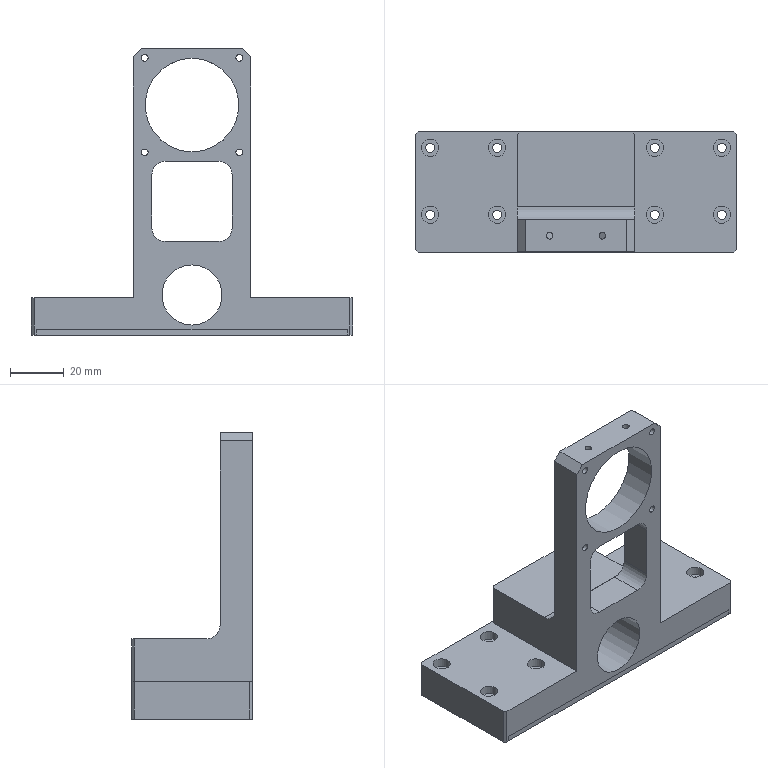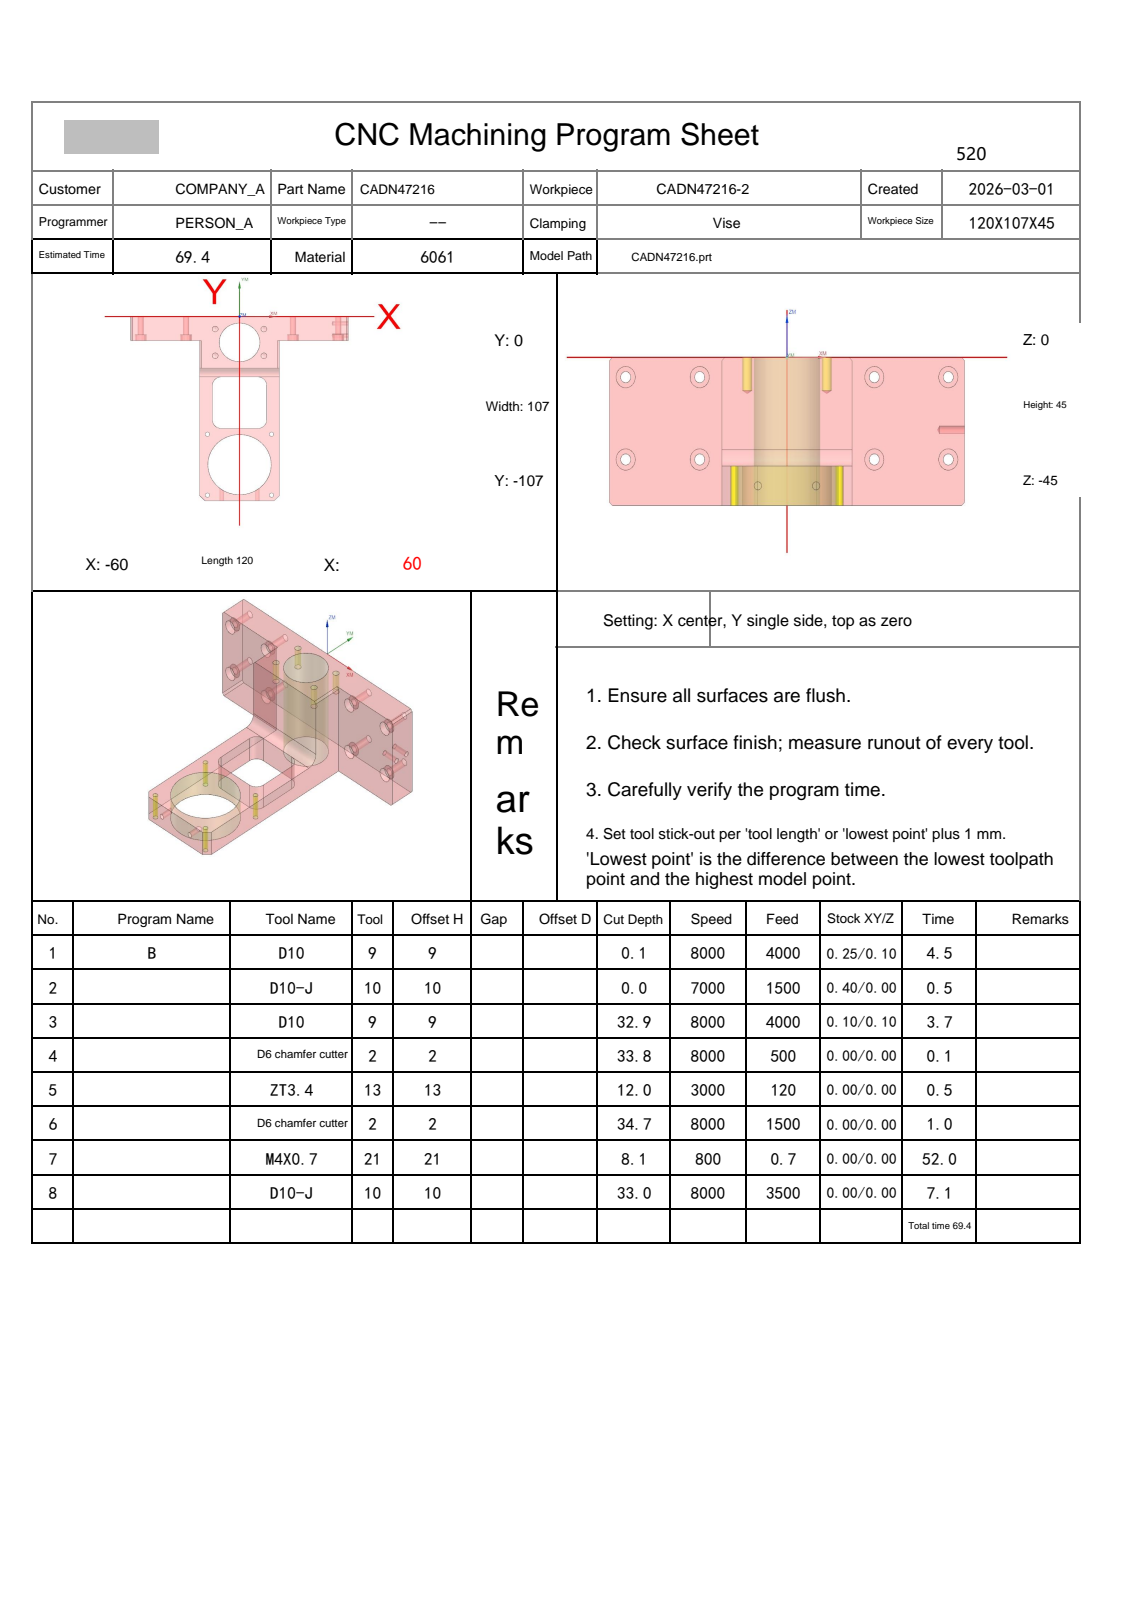NC program | NX | posted by the shop | part box 120 x 45 x 107 mm
Lines 1757 to 2535 of 8568:
N3 T09 M06
(D10  D=10. R=0. H=09 ce=0.10 di=0.10)
G00 G90 G54 X31.378 Y-24.062 M03 S8000
G43 H09 Z50.
M08
Z-14.45
G01 X31.287 Y-24.104 Z-15.075 F4000.
X31.196 Y-24.146 Z-15.322
X31.106 Y-24.188 Z-15.504
X31.015 Y-24.23 Z-15.65
X30.924 Y-24.273 Z-15.773
X30.834 Y-24.315 Z-15.878
X30.743 Y-24.357 Z-15.97
X30.652 Y-24.399 Z-16.05
X30.562 Y-24.441 Z-16.12
X30.471 Y-24.484 Z-16.182
X30.38 Y-24.526 Z-16.236
X30.29 Y-24.568 Z-16.283
X30.199 Y-24.61 Z-16.324
X30.108 Y-24.652 Z-16.358
X30.018 Y-24.695 Z-16.386
X29.927 Y-24.737 Z-16.41
X29.836 Y-24.779 Z-16.427
X29.746 Y-24.821 Z-16.44
X29.655 Y-24.863 Z-16.447
X29.564 Y-24.905 Z-16.45
X27.405 Y-25.91
G03 X27.113 Y-26.369 I.214 J-.458
G01 X27.151 Y-26.562
G02 X29.467 Y-30.08 I-25.429 J-19.261
X30.973 Y-36.095 I-14.623 J-6.857
X31.232 Y-44.397 I-132.782 J-8.303
X31.223 Y-46.009 I-133.041 J0.0
G01 X31.225 Y-102.469
G02 X28.237 Y-110.318 I-12.757 J.363
X23.784 Y-114.408 I-11.871 J8.455
X17.95 Y-115.972 I-6.708 J13.363
X9.211 Y-116.264 I-8.739 J130.435
X7.077 Y-116.247 I0.0 J130.728
G01 X-17.303 Y-116.232
G02 X-25.268 Y-113.271 I.206 J12.75
X-29.344 Y-108.898 I8.605 J12.105
X-30.935 Y-103.316 I12.645 J6.621
X-31.252 Y-95.378 I99.044 J7.938
X-31.242 Y-93.965 I99.361 J0.0
G01 X-31.225 Y-37.19
G02 X-31.229 Y-36.904 I11.714 J.286
X-29.463 Y-30.719 I11.718 J0.0
X-27.184 Y-28.116 I13.292 J-9.337
G01 X-27.1 Y-27.88
Y-26.52
X-27.126 Y-28.038
X-28.84 Y-31.056
G03 X-30.423 Y-37.625 I15.495 J-7.21
X-30.626 Y-46.505 I194. J-8.88
X-30.608 Y-49.142 I194.203 J0.0
G01 X-30.585 Y-96.082
G03 X-30.591 Y-96.853 I51.642 J-.771
X-30.097 Y-103.978 I51.647 J0.0
X-25.324 Y-112.093 I13.34 J2.385
X-17.597 Y-115.308 I8.755 J10.148
X-10.151 Y-115.615 I7.447 J90.294
X-8.726 Y-115.604 I0.0 J90.6
G01 X11.574 Y-115.579
G03 X12.22 Y-115.583 I.646 J46.187
X19.226 Y-115.049 I0.0 J46.192
X27.093 Y-110.328 I-2.634 J13.305
X30.314 Y-102.544 I-10.197 J8.777
X30.611 Y-95.169 I-91.526 J7.375
X30.6 Y-93.753 I-91.822 J0.0
G01 X30.561 Y-42.733
G03 X30.567 Y-41.955 I-52.094 J.778
X30.067 Y-34.756 I-52.1 J0.0
X27.429 Y-28.654 I-12.773 J-1.901
G02 X27.1 Y-28.125 I.757 J.838
G01 Y-26.525
X27.109 Y-28.284
G02 X28.595 Y-32.651 I-100.066 J-36.506
X29.677 Y-41.203 I-36.109 J-8.913
X29.793 Y-52.445 I-544.946 J-11.242
X29.789 Y-54.562 I-545.062 J0.0
G01 X29.778 Y-96.142
G02 X29.782 Y-96.738 I-41.25 J-.595
X29.28 Y-103.155 I-41.254 J0.0
X18.117 Y-114.102 I-13.308 J2.406
X10.092 Y-114.76 I-8.025 J48.608
G01 X9.834 Y-114.759
G02 X-.605 Y-114.831 I-10.439 J751.569
X-13.845 Y-114.715 I0.0 J751.641
X-20.222 Y-113.721 I.088 J21.521
X-29.054 Y-103.354 I4.381 J12.677
X-29.76 Y-95.187 I46.884 J8.167
X-29.759 Y-94.835 I47.59 J0.0
G01 X-29.809 Y-83.635
X-29.78 Y-42.775
G02 X-29.785 Y-42.143 I39.535 J.632
X-29.214 Y-35.448 I39.54 J0.0
X-27.14 Y-29.947 I23.047 J-5.549
G03 X-27.077 Y-28.644 I-13.57 J1.302
X-27.1 Y-27.857 I-13.632 J0.0
G02 X-27.077 Y-28.705 I-15.592 J-.848
X-27.165 Y-30.362 I-15.615 J0.0
G03 X-28.366 Y-34.989 I173.965 J-47.627
X-29.123 Y-43.529 I47.78 J-8.54
G01 X-29.122 Y-43.824
X-29.168 Y-53.664
X-29.144 Y-92.524
G03 X-29.148 Y-93.262 I66.05 J-.739
X-28.637 Y-101.462 I66.055 J0.0
X-25.247 Y-109.202 I14.471 J1.725
X-16.817 Y-113.605 I10.331 J9.509
X-8.943 Y-114.149 I7.873 J56.692
X-8.202 Y-114.144 I0.0 J57.236
X-.989 Y-114.192 I7.213 J546.31
X12.036 Y-114.036 I0.0 J546.357
X19.454 Y-112.945 I-.395 J28.436
X28.448 Y-102.635 I-4.112 J12.666
X29.124 Y-94.933 I-43.556 J7.702
X29.122 Y-94.515 I-44.232 J0.0
G01 X29.161 Y-84.915
X29.121 Y-45.735
G03 X29.125 Y-44.953 I-69.29 J.782
X28.545 Y-36.001 I-69.294 J0.0
X27.105 Y-30.369 I-36.876 J-6.426
G01 X27.1 Y-28.129
G03 X27.075 Y-29.766 I54.369 J-1.637
X27.105 Y-31.568 I54.394 J0.0
G02 X28.029 Y-39.059 I-149.321 J-22.233
X28.363 Y-50.799 I-206.184 J-11.741
X28.346 Y-53.452 I-206.518 J0.0
G01 X28.334 Y-93.032
G02 X28.337 Y-93.631 I-50.422 J-.599
X27.76 Y-101.242 I-50.426 J0.0
X23.057 Y-109.625 I-13.494 J2.06
X15.828 Y-112.669 I-9.501 J12.456
X7.016 Y-113.328 I-8.812 J58.609
X6.582 Y-113.326 I0.0 J59.267
X-.498 Y-113.39 I-7.08 J393.216
X-11.976 Y-113.222 I0.0 J393.28
X-19.119 Y-111.974 I.479 J23.804
X-27.181 Y-102.96 I4.572 J12.203
X-28.249 Y-94.649 I34.605 J8.668
X-28.376 Y-83.409 I496.508 J11.24
X-28.368 Y-80.57 I496.635 J0.0
G01 X-28.339 Y-45.55
G02 X-28.342 Y-44.949 I57.189 J.601
X-27.672 Y-36.225 I57.192 J0.0
G01 X-26.746 Y-31.943
G02 X-27.1 Y-30.285 I19.233 J4.973
G01 Y-29.805
X-27.101 Y-29.914
G03 X-26.721 Y-31.874 I5.242 J0.0
G02 X-26.697 Y-32.687 I-13.534 J-.813
X-26.925 Y-35.167 I-13.558 J0.0
G03 X-27.72 Y-47.475 I94.897 J-12.308
X-27.713 Y-48.652 I95.691 J0.0
G01 X-27.704 Y-89.592
G03 X-27.708 Y-90.402 I75.138 J-.81
X-27.176 Y-99.33 I75.143 J0.0
X-24.649 Y-106.431 I16.602 J1.908
X-16.627 Y-111.758 I10.889 J7.693
X-8.317 Y-112.653 I8.31 J38.132
G01 X-8.292
G03 X-.746 Y-112.743 I7.545 J316.058
X10.505 Y-112.543 I0.0 J316.148
X18.212 Y-111.254 I-.771 J28.298
X26.662 Y-101.992 I-4.196 J12.313
X27.62 Y-94.229 I-33.497 J8.077
X27.72 Y-84.554 I-469.811 J9.675
G01 X27.719 Y-83.589
X27.676 Y-47.37
Y-47.294
G03 X26.653 Y-32.982 I-100.698 J0.0
G02 X26.594 Y-32.506 I1.888 J.476
X26.882 Y-31.488 I1.947 J0.0
G01 X27.096 Y-30.307
G02 X26.563 Y-32.204 I-5.193 J.436
G03 X26.311 Y-34.555 I10.823 J-2.351
X26.367 Y-35.665 I11.076 J0.0
G02 X26.918 Y-52.661 I-261.615 J-16.996
X26.906 Y-55.176 I-262.167 J0.0
G01 X26.895 Y-90.116
G02 X26.898 Y-90.756 I-61.402 J-.64
X26.346 Y-98.97 I-61.405 J0.0
X23.294 Y-106.288 I-14.97 J1.948
X15.946 Y-110.754 I-10.539 J9.062
X7.148 Y-111.813 I-9.137 J38.832
X-.509 Y-111.938 I-7.657 J234.058
X-10.527 Y-111.724 I0.0 J234.183
X-17.878 Y-110.295 I.828 J23.886
X-25.465 Y-101.923 I4.841 J12.011
X-26.732 Y-93.966 I30.346 J8.911
X-26.948 Y-81.79 I341.949 J12.176
X-26.927 Y-77.969 I342.165 J0.0
G01 X-26.896 Y-47.429
G02 X-26.069 Y-34.589 I120.822 J-1.336
G03 X-26.027 Y-33.866 I-6.234 J.723
X-26.084 Y-33.027 I-6.276 J0.0
G02 X-26.745 Y-31.794 I3.668 J2.764
G03 X-26.046 Y-33.053 I3.428 J1.083
G02 X-25.721 Y-35.362 I-8.05 J-2.31
X-25.757 Y-36.145 I-8.374 J0.0
G03 X-26.3 Y-53.002 I261.501 J-16.856
X-26.286 Y-55.747 I262.044 J0.0
G01 X-26.257 Y-87.727
G03 X-26.259 Y-88.371 I74.064 J-.644
X-25.679 Y-97.622 I74.067 J0.0
X-23.093 Y-104.874 I17.286 J2.078
X-15.476 Y-110.112 I10.873 J7.652
X-7.403 Y-111.166 I8.526 J33.889
X-.584 Y-111.291 I6.818 J185.68
X9.71 Y-111.005 I0.0 J185.805
X17.432 Y-109.401 I-1.208 J25.194
X25.033 Y-100.747 I-4.954 J12.016
X26.154 Y-92.605 I-32.369 J8.606
X26.285 Y-82.334 I-401.884 J10.27
X26.277 Y-79.806 I-402.015 J0.0
G01 X26.231 Y-48.546
G03 X25.76 Y-35.75 I-378.609 J-7.53
G02 X25.749 Y-35.228 I11.449 J.522
X25.926 Y-33.218 I11.46 J0.0
G03 X26.581 Y-32.164 I-2.862 J2.509
G02 X25.876 Y-33.258 I-3.048 J1.191
G03 X25.242 Y-36.226 I6.634 J-2.968
G01 Y-36.258
G03 X25.218 Y-38.769 I134.464 J-2.511
X25.359 Y-44.915 I134.487 J0.0
G02 X25.471 Y-57.51 I-710.16 J-12.595
X25.468 Y-59.234 I-710.272 J0.0
G01 X25.448 Y-88.174
G02 X25.45 Y-88.756 I-60.973 J-.582
X24.831 Y-97.424 I-60.976 J0.0
X21.912 Y-104.527 I-15.373 J2.166
X14.597 Y-109.167 I-10.771 J8.895
X5.895 Y-110.335 I-9.331 J36.5
X-.49 Y-110.476 I-6.385 J144.542
X-9.617 Y-110.188 I0.0 J144.683
X-16.913 Y-108.5 I1.246 J21.999
X-23.826 Y-100.666 I5.479 J11.803
X-25.267 Y-92.252 I29.65 J9.407
X-25.498 Y-81.145 I266.483 J11.107
X-25.485 Y-78.495 I266.714 J0.0
G01 X-25.458 Y-49.235
G02 X-25.023 Y-36.981 I348.594 J-6.226
G03 X-25.003 Y-36.336 I-10.259 J.646
X-25.29 Y-33.925 I-10.279 J0.0
G02 X-26.119 Y-32.943 I11.749 J10.759
G03 X-25.298 Y-33.859 I2.829 J1.707
G02 X-24.622 Y-36.586 I-5.315 J-2.766
X-24.577 Y-39.34 I-84.448 J-2.754
X-24.703 Y-43.961 I-84.493 J0.0
G03 X-24.847 Y-56.677 I562.086 J-12.716
X-24.846 Y-58.04 I562.23 J0.0
G01 X-24.818 Y-85.22
G03 X-24.822 Y-85.952 I81.406 J-.732
X-24.248 Y-95.597 I81.41 J0.0
X-21.769 Y-102.983 I18.506 J2.103
X-14.074 Y-108.547 I11.147 J7.313
X-5.615 Y-109.708 I8.905 J33.5
X-.457 Y-109.82 I5.158 J118.314
X9.093 Y-109.434 I0.0 J118.426
X16.725 Y-107.476 I-1.642 J22.251
X23.504 Y-99.212 I-5.91 J11.761
X24.698 Y-90.839 I-32.631 J8.924
X24.849 Y-79.789 I-403.753 J11.05
X24.835 Y-76.441 I-403.904 J0.0
G01 X24.787 Y-49.261
G02 X24.599 Y-37.857 I604.945 J15.677
X24.595 Y-37.57 I11.482 J.286
X25.165 Y-33.998 I11.486 J0.0
X25.574 Y-33.638 I4.249 J-4.413
G01 X25.969 Y-33.135
G02 X25.154 Y-33.963 I-2.324 J1.471
G03 X24.178 Y-36.645 I4.634 J-3.204
X23.875 Y-41.89 I45.177 J-5.245
X23.911 Y-43.708 I45.481 J0.0
G02 X24.038 Y-58.218 I-828.198 J-14.51
X24.029 Y-62.016 I-828.325 J0.0
G01 X24.008 Y-85.836
G02 X24.011 Y-86.513 I-65.707 J-.677
X23.384 Y-95.567 I-65.711 J0.0
X20.563 Y-102.73 I-16.032 J2.177
X13.204 Y-107.605 I-11.022 J8.647
X4.433 Y-108.863 I-9.533 J35.259
X-.505 Y-108.995 I-4.938 J92.508
X-9.072 Y-108.598 I0.0 J92.639
X-16.39 Y-106.443 I1.659 J19.135
X-22.417 Y-98.791 I6.81 J11.565
X-23.814 Y-90.452 I31.062 J9.49
X-24.066 Y-78.199 I298.074 J12.253
X-24.045 Y-74.696 I298.326 J0.0
G01 X-24.013 Y-49.916
G03 X-23.807 Y-38.735 I-925.837 J22.631
X-23.804 Y-38.46 I-12.436 J.275
X-24.358 Y-34.789 I-12.439 J0.0
X-24.59 Y-34.382 I-3.237 J-1.577
G01 X-25.355 Y-33.803
G02 X-24.339 Y-34.646 I-2.322 J-3.835
X-23.396 Y-37.976 I-6.535 J-3.648
X-23.246 Y-42.329 I-63.133 J-4.353
X-23.287 Y-44.586 I-63.283 J0.0
G03 X-23.411 Y-58.33 I759.267 J-13.744
X-23.405 Y-61.304 I759.391 J0.0
G01 X-23.369 Y-83.844
G03 X-23.371 Y-84.392 I75.82 J-.548
X-22.732 Y-94.216 I75.822 J0.0
X-20.159 Y-101.56 I18.414 J2.33
X-12.353 Y-107.09 I11.267 J7.629
X-3.892 Y-108.239 I8.907 J33.843
X-.273 Y-108.323 I3.619 J77.808
X8.726 Y-107.802 I0.0 J77.892
X16.276 Y-105.337 I-2.114 J19.269
X22.048 Y-97.489 I-7.261 J11.387
X23.249 Y-89.034 I-33.662 J9.09
X23.405 Y-78.246 I-371.026 J10.788
X23.394 Y-75.356 I-371.183 J0.0
G01 X23.351 Y-50.496
G02 X23.277 Y-44.774 I218.888 J5.722
X23.342 Y-39.421 I218.963 J0.0
X24.112 Y-35.088 I13.883 J-.232
X24.589 Y-34.382 I1.326 J-.382
G01 X25.228 Y-33.9
G03 X24.015 Y-34.917 I2.851 J-4.631
X22.849 Y-38.483 I7.259 J-4.348
X22.508 Y-44.673 I56.01 J-6.191
X22.525 Y-46.065 I56.351 J0.0
G01 X22.589 Y-63.407
X22.567 Y-83.707
G02 X22.57 Y-84.403 I-69.97 J-.696
X21.953 Y-93.679 I-69.973 J0.0
X19.211 Y-100.952 I-16.807 J2.182
X11.719 Y-106.081 I-11.283 J8.445
X2.799 Y-107.387 I-9.565 J34.207
X-.603 Y-107.483 I-3.402 J60.372
X-8.853 Y-106.917 I0.0 J60.468
X-16.187 Y-104.04 I2.183 J16.351
X-21.097 Y-96.674 I8.764 J11.162
X-22.391 Y-88.231 I34.397 J9.592
X-22.614 Y-76.976 I283.942 J11.255
X-22.604 Y-74.554 I284.165 J0.0
G01 X-22.569 Y-50.414
G03 X-22.486 Y-44.47 I-212.675 J5.945
X-22.535 Y-39.873 I-212.758 J0.0
X-23.357 Y-35.495 I-12.83 J-.144
X-23.927 Y-34.676 I-1.738 J-.6
G01 X-24.526 Y-34.431
G02 X-23.026 Y-35.731 I-.526 J-2.122
X-22.022 Y-40.146 I-11.066 J-4.837
X-21.873 Y-46.567 I-138.264 J-6.421
X-21.928 Y-50.459 I-138.413 J0.0
G01 X-21.962 Y-75.719
G03 X-21.976 Y-78.071 I190.046 J-2.352
X-21.643 Y-89.312 I190.061 J0.0
X-19.98 Y-97.431 I27.733 J1.451
X-11.038 Y-105.518 I12.608 J4.955
X-2.27 Y-106.742 I8.918 J31.871
X.018 Y-106.793 I2.288 J50.999
X8.884 Y-106.017 I0.0 J51.05
X16.193 Y-102.768 I-2.787 J16.116
X20.774 Y-95.165 I-9.455 J10.878
X21.837 Y-86.368 I-39.499 J9.238
X21.96 Y-75.205 I-506.71 J11.163
X21.952 Y-72.369 I-506.833 J0.0
G01 X21.895 Y-48.141
G02 X21.867 Y-46.109 I73.298 J2.032
X22.183 Y-39.304 I73.326 J0.0
X23.381 Y-35.254 I10.2 J-.813
X23.87 Y-34.699 I1.736 J-1.04
G01 X24.524 Y-34.432
G03 X22.583 Y-36.13 I.746 J-2.811
X21.385 Y-40.932 I12.609 J-5.695
X21.092 Y-48.871 I107.46 J-7.939
X21.119 Y-51.261 I107.753 J0.0
G01 X21.132 Y-81.001
G02 X21.138 Y-81.954 I-80.385 J-.953
X20.555 Y-91.617 I-80.391 J0.0
X18.093 Y-98.831 I-18.124 J2.159
X10.359 Y-104.523 I-11.671 J7.758
X1.207 Y-105.875 I-9.405 J32.001
X-.77 Y-105.923 I-1.977 J40.635
X-8.741 Y-105.135 I0.0 J40.683
X-16.35 Y-100.983 I2.782 J14.149
X-20.063 Y-93.431 I12.312 J10.741
X-21.047 Y-84.138 I48.525 J9.835
X-21.188 Y-67.721 I956.12 J16.417
X-21.164 Y-60.959 I956.261 J0.0
G01 X-21.112 Y-43.698
G03 X-21.11 Y-43.341 I-26.25 J.358
X-21.773 Y-37.476 I-26.253 J0.0
X-23. Y-35.034 I-5.305 J-1.135
G01 X-23.899 Y-34.687
G03 X-23.052 Y-34.974 I1.537 J3.14
G02 X-21.629 Y-36.883 I-2.178 J-3.111
X-20.603 Y-42.454 I-16.703 J-5.955
X-20.47 Y-49.82 I-203.908 J-7.367
X-20.506 Y-53.657 I-204.041 J0.0
G01 X-20.496 Y-79.157
G03 X-20.499 Y-79.97 I88.826 J-.812
X-19.883 Y-90.413 I88.83 J0.0
X-17.44 Y-97.989 I20.158 J2.317
X-9.2 Y-104.104 I11.763 J7.242
X-.759 Y-105.203 I8.441 J31.863
X.226 Y-105.189 I0.0 J32.962
X.66 Y-105.192 I.434 J32.338
X9.703 Y-103.901 I0.0 J32.341
X19.088 Y-94.318 I-3.956 J13.26
X20.334 Y-85.95 I-33.57 J9.277
X20.527 Y-74.575 I-335.129 J11.375
X20.511 Y-71.312 I-335.322 J0.0
G01 X20.5 Y-46.548
G02 X20.497 Y-46.102 I40.216 J.447
X21.156 Y-38.85 I40.219 J0.0
X22.705 Y-35.284 I8.113 J-1.403
X23.305 Y-34.93 I.687 J-.479
G01 X23.75 Y-34.748
G02 X23.003 Y-34.976 I-1.074 J2.185
G03 X21.311 Y-36.932 I1.966 J-3.412
X20.012 Y-42.294 I15.2 J-6.521
X19.676 Y-50.819 I107.982 J-8.525
X19.691 Y-52.634 I108.318 J0.0
G01 X19.685 Y-79.709
G02 X19.688 Y-80.44 I-76.953 J-.731
X19.082 Y-90.083 I-76.957 J0.0
X16.418 Y-97.563 I-17.99 J2.192
X8.641 Y-103.079 I-11.653 J8.19
X-.185 Y-104.308 I-8.827 J31.067
X-1.884 Y-104.263 I0.0 J32.297
X-10.172 Y-102.683 I.244 J23.804
X-17.828 Y-94.436 I5.309 J12.605
X-19.407 Y-86.131 I29.405 J9.894
X-19.728 Y-75.01 I192.621 J11.121
X-19.719 Y-73.098 I192.942 J0.0
G01 X-19.706 Y-46.17
G03 X-19.703 Y-45.731 I-35.802 J.439
X-20.369 Y-38.858 I-35.805 J0.0
X-21.989 Y-35.384 I-7.476 J-1.371
X-22.482 Y-35.037 I-.998 J-.895
G01 X-23.275 Y-34.934
G02 X-22.136 Y-35.159 I-.043 J-3.205
X-20.356 Y-37.61 I-2.921 J-3.994
X-19.238 Y-43.534 I-18.919 J-6.639
X-19.048 Y-51.253 I-157.167 J-7.719
X-19.065 Y-53.526 I-157.356 J0.0
G01 X-19.055 Y-77.186
G03 X-19.059 Y-77.998 I93.386 J-.812
X-18.464 Y-88.523 I93.389 J0.0
X-16.091 Y-96.203 I21.03 J2.291
X-7.775 Y-102.555 I11.9 J6.96
X-.095 Y-103.568 I7.68 J28.609
X3.567 Y-103.341 I0.0 J29.622
X11.463 Y-100.923 I-1.669 J19.549
X17.558 Y-92.932 I-7.257 J11.854
X18.879 Y-84.417 I-32.866 J9.46
X19.083 Y-73.332 I-301.377 J11.085
X19.07 Y-70.5 I-301.58 J0.0
G01 X19.079 Y-48.866
G02 X19.077 Y-48.403 I49.728 J.463
X19.755 Y-40.219 I49.73 J0.0
X21.419 Y-35.968 I10.569 J-1.687
X22.459 Y-35.04 I2.162 J-1.378
G01 X23.094 Y-34.958
G03 X20.864 Y-36.216 I.047 J-2.689
X19.044 Y-40.749 I9.22 J-6.332
X18.301 Y-49.394 I49.937 J-8.645
G01 X18.302 Y-49.673
G03 X18.247 Y-58.853 I761.188 J-9.18
X18.267 Y-64.451 I761.243 J0.0
G02 X18.294 Y-69.613 I-503.362 J-5.162
X18.112 Y-83.149 I-503.388 J0.0
X16.945 Y-91.609 I-36.774 J.761
X7.306 Y-101.498 I-13.529 J3.546
X-.236 Y-102.62 I-7.542 J24.777
X-7.371 Y-101.618 I0.0 J25.9
X-16.337 Y-92.921 I4.031 J13.126
X-17.978 Y-84.221 I29.99 J10.163
X-18.29 Y-72.739 I211.04 J11.482
X-18.279 Y-70.547 I211.352 J0.0
G01 X-18.29 Y-48.095
G03 X-18.289 Y-47.693 I-42.527 J.402
X-19.011 Y-39.886 I-42.529 J0.0
X-20.87 Y-35.726 I-9.189 J-1.61
X-21.748 Y-35.1 I-1.339 J-.949
G01 X-22.478 Y-35.038
X-21.589 Y-35.108
G02 X-19.716 Y-36.891 I-1.523 J-3.474
X-18.08 Y-42.388 I-13.063 J-6.881
X-17.627 Y-50.932 I-80.479 J-8.544
X-17.636 Y-52.116 I-80.931 J0.0
G01 X-17.613 Y-75.512
G03 X-17.616 Y-76.294 I93.163 J-.782
X-17.007 Y-86.929 I93.167 J0.0
X-14.678 Y-94.535 I21.357 J2.381
X-5.848 Y-101.112 I11.968 J6.85
X-.111 Y-101.833 I5.736 J22.468
X7.848 Y-100.424 I0.0 J23.188
X15.986 Y-91.684 I-5.008 J12.821
X17.394 Y-83.428 I-30.581 J9.464
X17.645 Y-72.073 I-256.247 J11.354
X17.628 Y-69.112 I-256.498 J0.0
G02 X17.601 Y-62.256 I880.041 J6.856
X17.712 Y-48.304 I880.068 J0.0
X18.647 Y-40.089 I39.59 J-.346
X20.661 Y-35.878 I9.721 J-2.06
X21.749 Y-35.1 I1.781 J-1.341
G01 X22.397 Y-35.048
G03 X21.405 Y-35.152 I1.277 J-16.974
X19.228 Y-37.248 I1.912 J-4.164
X17.441 Y-42.982 I14.381 J-7.627
X16.843 Y-52.577 I76.702 J-9.595
X16.846 Y-53.239 I77.3 J0.0
G01 X16.793 Y-76.773
G02 X16.796 Y-77.357 I-71.847 J-.584
X16.115 Y-87.221 I-71.85 J0.0
X13.33 Y-94.656 I-17.75 J2.41
X5.086 Y-100.136 I-11.492 J8.348
X-.154 Y-100.827 I-5.239 J19.516
X-7.036 Y-99.619 I0.0 J20.207
X-14.763 Y-91.627 I5.032 J12.598
X-16.49 Y-83.112 I28.367 J10.185
X-16.847 Y-71.664 I183.578 J11.448
X-16.836 Y-69.679 I183.935 J0.0
G01 X-16.858 Y-50.404
G03 X-16.856 Y-49.901 I-54.056 J.503
X-17.555 Y-41.231 I-54.059 J0.0
X-19.484 Y-36.302 I-11.976 J-1.843
X-20.892 Y-35.106 I-2.626 J-1.666
G01 X-21.728 Y-35.1
G02 X-21.358 Y-35.08 I.371 J-3.389
X-20.563 Y-35.174 I0.0 J-3.409
X-18.45 Y-37.326 I-2.192 J-4.265
X-16.715 Y-43.205 I-14.802 J-7.564
X-16.194 Y-52.743 I-87.013 J-9.539
X-16.203 Y-54.039 I-87.534 J0.0
G01 X-16.162 Y-74.655
G03 X-16.164 Y-75.221 I82.489 J-.566
X-15.469 Y-85.904 I82.491 J0.0
X-12.884 Y-93.512 I19.994 J2.552
X-3.615 Y-99.63 I11.491 J7.328
X-.05 Y-99.986 I3.565 J17.663
X7.989 Y-98.094 I0.0 J18.019
X14.568 Y-89.981 I-6.619 J12.093
X15.976 Y-81.32 I-32.198 J9.68
X16.199 Y-70.301 I-273.167 J11.019
X16.186 Y-67.723 I-273.389 J0.0
G02 X16.16 Y-62.31 I551.801 J5.413
X16.323 Y-48.901 I551.827 J0.0
X17.46 Y-40.269 I38.09 J-.626
X19.701 Y-35.949 I9.979 J-2.435
X20.954 Y-35.1 I2.193 J-1.888
G01 X21.674
G03 X21.31 Y-35.076 I-.364 J-2.796
X19.196 Y-36.03 I0.0 J-2.819
X16.784 Y-40.511 I7.671 J-7.019
X15.573 Y-49.013 I36.114 J-9.48
X15.361 Y-61.898 I391.583 J-12.885
X15.386 Y-66.315 I391.795 J0.0
G02 X15.405 Y-69.497 I-267.052 J-3.181
X15.152 Y-81.111 I-267.071 J0.0
X13.761 Y-89.289 I-31.629 J1.173
X3.101 Y-98.566 I-12.968 J4.139
X-.134 Y-98.906 I-3.235 J15.205
X-7.385 Y-97.111 I0.0 J15.545
X-13.418 Y-89.735 I6.9 J11.798
X-15.073 Y-81.121 I29.874 J10.206
X-15.414 Y-68.965 I216.42 J12.156
X-15.398 Y-66.328 I216.761 J0.0
G03 X-15.375 Y-61.217 I-573.037 J5.111
X-15.506 Y-48.979 I-573.06 J0.0
X-16.559 Y-40.425 I-38.998 J-.462
X-18.878 Y-35.876 I-10.133 J-2.3
X-20.013 Y-35.1 I-1.949 J-1.632
G01 X-20.893
G02 X-20.495 Y-35.081 I.398 J-4.143
X-19.651 Y-35.167 I0.0 J-4.163
X-17.424 Y-37.278 I-2.138 J-4.487
X-15.462 Y-43.171 I-14.186 J-7.996
X-14.781 Y-53.15 I-72.808 J-9.979
X-14.784 Y-53.827 I-73.489 J0.0
G01 X-14.714 Y-73.377
X-14.715 Y-73.767
G03 X-14.004 Y-84.385 I79.599 J0.0
X-11.426 Y-91.903 I19.877 J2.616
X-.838 Y-97.943 I11.001 J6.984
X.161 Y-97.979 I.999 J13.711
X9.591 Y-94.235 I0.0 J13.748
X13.54 Y-86.936 I-11.015 J10.677
X14.627 Y-77.577 I-43.6 J9.81
X14.768 Y-62.641 I-794.205 J14.937
X14.753 Y-57.784 I-794.345 J0.0
G02 X14.744 Y-56.338 I115.333 J1.446
X15.267 Y-45.366 I115.342 J0.0
X17.082 Y-38.334 I22.245 J-1.992
X19.685 Y-35.244 I6.396 J-2.745
G01 X20.061 Y-35.1
X20.941
G03 X20.514 Y-35.079 I-.428 J-4.431
X19.525 Y-35.191 I0.0 J-4.451
X16.971 Y-37.547 I2.273 J-5.027
X14.822 Y-43.744 I15.257 J-8.761
X14.008 Y-54.396 I69.498 J-10.671
X13.922 Y-66.982 I920.951 J-12.586
X13.931 Y-71.117 I921.037 J0.0
G02 X13.937 Y-72.224 I-105.855 J-1.107
X13.448 Y-82.381 I-105.861 J0.0
X11.295 Y-90.038 I-21.566 J1.933
X-.004 Y-96.804 I-11.299 J6.051
X-2.463 Y-96.566 I0.0 J12.817
X-11.369 Y-89.494 I2.336 J12.085
X-13.466 Y-81.236 I23.3 J10.311
X-13.953 Y-69.972 I130.068 J11.264
X-13.945 Y-68.61 I130.555 J0.0
G03 X-13.935 Y-64.716 I-758.668 J3.894
X-14.066 Y-50.646 I-758.678 J0.0
X-15.114 Y-41.395 I-45.76 J-.5
X-17.455 Y-36.315 I-12.391 J-2.632
X-18.964 Y-35.111 I-3.227 J-2.495
G01 X-19.985 Y-35.1
G02 X-19.564 Y-35.082 I.422 J-4.988
X-18.674 Y-35.162 I0.0 J-5.006
X-16.231 Y-37.445 I-2.23 J-4.834
X-14.103 Y-43.749 I-15.209 J-8.646
X-13.357 Y-54.255 I-73.58 J-10.506
G01 X-13.358 Y-54.641
X-13.262 Y-72.343
Y-72.493
G03 X-12.523 Y-82.948 I74.348 J0.0
X-9.846 Y-90.429 I19.086 J2.611
X.036 Y-95.776 I9.882 J6.459
X10.581 Y-89.278 I0.0 J11.805
X12.801 Y-81.389 I-19.962 J9.876
X13.3 Y-70.869 I-110.71 J10.52
X13.292 Y-69.565 I-111.208 J0.0
G02 X13.278 Y-65.719 I534.499 J3.846
X13.467 Y-51.539 I534.513 J0.0
X14.664 Y-41.872 I46.768 J-.884
X17.199 Y-36.506 I13.226 J-2.968
X19.08 Y-35.1 I3.352 J-2.522
G01 X19.96
G03 X19.529 Y-35.077 I-.431 J-4.071
X18.403 Y-35.235 I0.0 J-4.094
X15.739 Y-37.769 I2.721 J-5.528
X13.436 Y-44.445 I16.534 J-9.44
X12.572 Y-55.757 I74.228 J-11.357
G01 X12.441 Y-73.282
Y-73.31
G02 X11.657 Y-82.999 I-60.236 J0.0
X8.723 Y-90.107 I-16.355 J2.592
X.115 Y-94.437 I-8.608 J6.391
X-6.275 Y-92.324 I0.0 J10.721
X-10.817 Y-85.529 I8.587 J10.656
X-12.251 Y-76.87 I33.79 J10.041
X-12.535 Y-64.158 I283.678 J12.712
X-12.518 Y-61.073 I283.963 J0.0
G03 X-12.504 Y-58.874 I-165.66 J2.2
X-12.906 Y-47.344 I-165.675 J0.0
X-14.558 Y-39.432 I-28.612 J-1.847
X-17.2 Y-35.543 I-8.745 J-3.099
X-17.992 Y-35.1 I-1.461 J-1.682
G01 X-18.952
G02 X-18.526 Y-35.081 I.426 J-4.858
X-17.627 Y-35.165 I0.0 J-4.876
X-15.217 Y-37.296 I-2.193 J-4.907
X-12.888 Y-43.484 I-14.4 J-8.952
X-11.96 Y-54.044 I-62.768 J-10.841
X-11.843 Y-68.35 I-877.91 J-14.307
G01 Y-69.071
G03 X-11.846 Y-69.751 I89.292 J-.68
X-11.189 Y-80.564 I89.294 J0.0
X-8.774 Y-88.055 I20.139 J2.356
X.163 Y-93.292 I8.938 J5.009
G01 X.185
G03 X8.754 Y-88.164 I-.368 J10.338
X11.177 Y-81.007 I-16.46 J9.562
X11.824 Y-71.166 I-74.547 J9.842
G01 X11.823 Y-70.796
G02 X12.008 Y-53.435 I828.875 J-.13
X13.162 Y-42.989 I55.042 J-.798
X15.697 Y-37.034 I15.843 J-3.227
X17.992 Y-35.111 I4.569 J-3.12
G01 X18.931 Y-35.1
G03 X18.496 Y-35.077 I-.435 J-4.101
X17.352 Y-35.239 I0.0 J-4.124
X14.551 Y-37.876 I2.831 J-5.812
X12.112 Y-44.741 I17.08 J-9.935
X11.149 Y-56.41 I73.295 J-11.92
G01 X10.979 Y-72.491
G02 X10.11 Y-81.797 I-52.41 J.197
X7.207 Y-88.333 I-14.829 J2.674
X.19 Y-91.758 I-7.018 J5.477
X-3.328 Y-91.034 I0.0 J8.902
X-8.649 Y-85.493 I4.738 J9.875
X-10.574 Y-77.846 I22.366 J9.696
X-11.06 Y-67.116 I118.279 J10.73
X-11.057 Y-66.261 I118.764 J0.0
G03 X-11.048 Y-63.851 I-325.637 J2.41
X-11.321 Y-50.502 I-325.646 J0.0
X-12.754 Y-41.171 I-40.258 J-1.405
X-15.499 Y-36.093 I-12.071 J-3.244
X-16.925 Y-35.1 I-2.55 J-2.142
G01 X-17.965
G02 X-17.497 Y-35.079 I.468 J-5.311
X-16.555 Y-35.163 I0.0 J-5.332
X-14.044 Y-37.352 I-2.249 J-5.115
X-11.566 Y-43.763 I-14.888 J-9.437
X-10.536 Y-54.777 I-63.182 J-11.465
X-10.373 Y-69.322 I-978.625 J-18.261
G01 Y-69.406
G03 X-9.597 Y-79.683 I68.491 J0.0
X-7.123 Y-86.394 I17.236 J2.543
X-.286 Y-90.43 I7.316 J4.585
G01 X-.235
G03 X6.94 Y-86.664 I0.0 J8.716
X9.635 Y-79.788 I-13.464 J9.244
X10.366 Y-70.19 I-62.65 J9.598
G01 Y-70.065
G02 X10.605 Y-53.78 I709.176 J-2.293
X11.872 Y-43.188 I54.411 J-1.138
X14.541 Y-37.094 I16.338 J-3.522
X16.884 Y-35.12 I4.955 J-3.503
G01 X17.947 Y-35.1
G03 X17.481 Y-35.077 I-.465 J-4.726
X16.318 Y-35.222 I0.0 J-4.749
X13.481 Y-37.768 I2.723 J-5.888
X10.842 Y-44.723 I16.747 J-10.332
X9.749 Y-56.201 I67.778 J-12.245
X9.552 Y-70.186 I941.188 J-20.257
G02 X8.744 Y-79.579 I-55.119 J.012
X6.189 Y-85.643 I-14.151 J2.392
X.32 Y-88.621 I-5.869 J4.295
X-4.553 Y-86.747 I0.0 J7.272
X-8.103 Y-81.029 I8.172 J9.036
X-9.389 Y-72.911 I32.641 J9.331
X-9.678 Y-58.697 I349.678 J14.214
G01 Y-58.087
X-9.677 Y-57.83
G03 X-10.439 Y-45.965 I-92.742 J0.0
X-12.682 Y-38.441 I-23.333 J-2.858
X-15.591 Y-35.171 I-7.1 J-3.388
X-16.441 Y-35.076 I-.85 J-3.746
X-16.872 Y-35.1 I0.0 J-3.842
G02 X-16.413 Y-35.082 I.459 J-6.014
X-15.47 Y-35.156 I0.0 J-6.032
X-12.814 Y-37.458 I-2.279 J-5.314
X-10.251 Y-43.966 I-15.472 J-9.851
X-9.123 Y-55.118 I-62.235 J-11.93
G01 X-8.88 Y-69.578
G03 X-7.917 Y-78.793 I48.468 J.41
X-5.285 Y-84.489 I13.187 J2.635
X-.12 Y-86.971 I5.166 J4.135
X4.207 Y-85.36 I0.0 J6.617
X7.676 Y-79.791 I-7.312 J8.42
X8.819 Y-71.651 I-33.06 J8.789
X9.09 Y-57.237 I-901.386 J24.158
G02 X10.125 Y-45.393 I75.586 J-.638
X12.716 Y-38.081 I21.371 J-3.46
X15.687 Y-35.157 I6.538 J-3.673
X16.463 Y-35.081 I.776 J-3.937
X16.851 Y-35.1 I0.0 J-4.013
G03 X16.387 Y-35.077 I-.464 J-4.771
X15.203 Y-35.226 I0.0 J-4.794
X12.259 Y-37.86 I2.823 J-6.117
X9.52 Y-44.934 I17.244 J-10.743
X8.342 Y-56.385 I66.4 J-12.619
G01 X8.071 Y-69.808
G02 X7.123 Y-78.138 I-40.075 J.344
X4.524 Y-83.13 I-10.395 J2.24
X.554 Y-84.728 I-3.969 J4.131
X-2.492 Y-83.851 I0.0 J5.729
X-6.454 Y-78.879 I5.11 J8.136
X-7.885 Y-71.604 I24.205 J8.542
X-8.247 Y-58.582 I234.751 J13.03
G03 X-9.091 Y-46.232 I-91.649 J-.066
X-11.41 Y-38.601 I-24.212 J-3.19
X-14.422 Y-35.192 I-7.483 J-3.577
G01 X-14.692 Y-35.1
X-15.812
G02 X-15.329 Y-35.083 I.483 J-6.844
X-14.342 Y-35.154 I0.0 J-6.861
X-11.773 Y-37.274 I-2.17 J-5.244